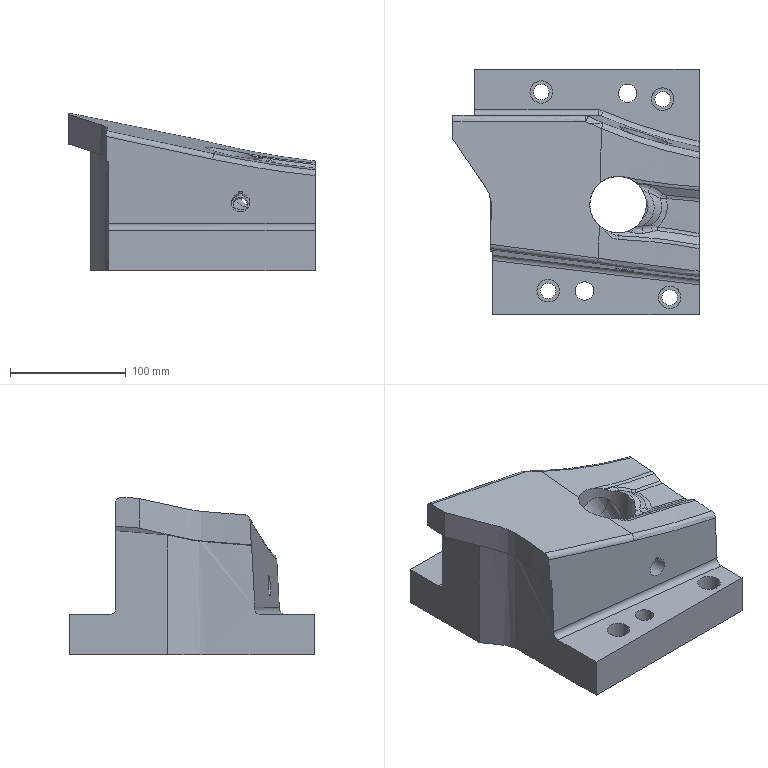Part | NX | features solid 2 | 1 solid | 73 faces | box 212.787 x 212 x 136.428 mm | volume 2725764 mm3 | spline 31 | cylinder 23 | plane 19 | commonest cylinder face diameters 13.5 x4 19.5 x4 10 x3 4 x2 16 x2 1640 x2